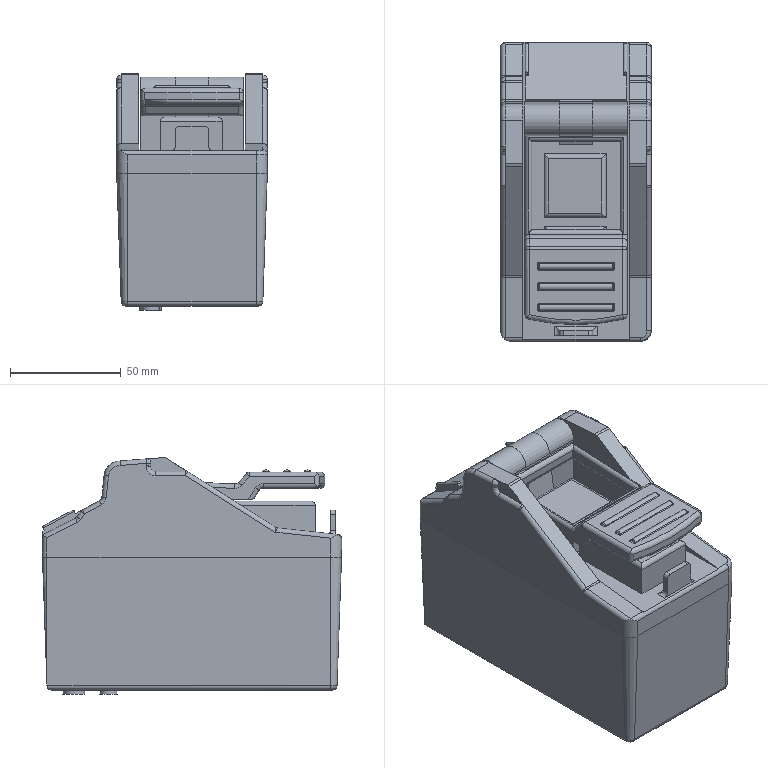Part | STEP file | DEWALT-DWE7492-B22 | 1 solid | 232 faces | box 68 x 135 x 106.953 mm | volume 732331 mm3 | cylinder 99 | plane 88 | torus 21 | sphere 10 | spline 8 | cone 4 | other 2 | commonest cylinder face diameters 4 x73 1 x6 1.5 x6 3.25 x3 10 x3 14.487 x3